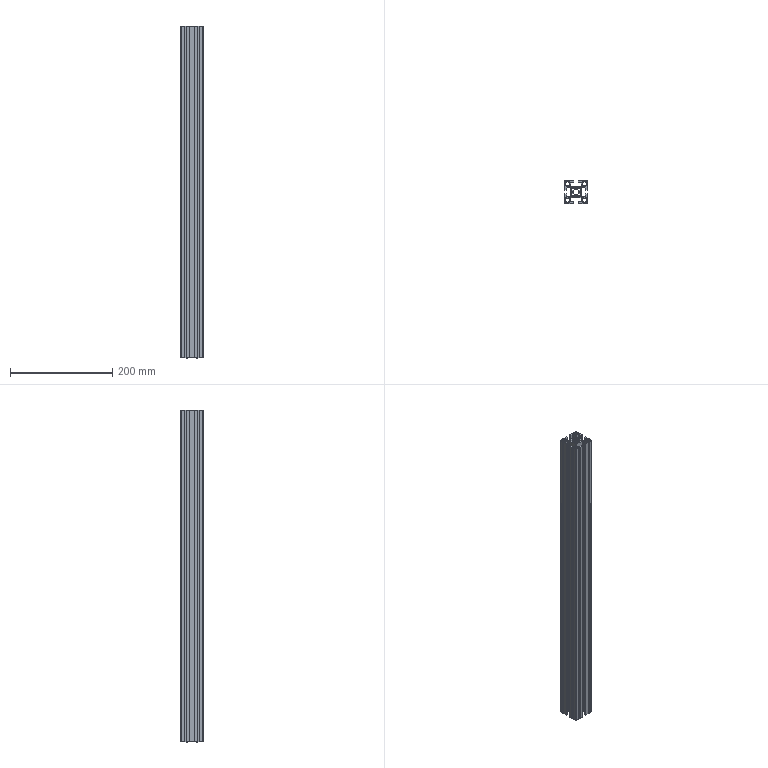Part | STEP file | 4545-650 Al (PC rack 1) | 1 solid | 262 faces | box 45 x 45 x 650 mm | volume 451001 mm3 | plane 186 | cylinder 76 | commonest cylinder face diameters 2 x44 8 x20 12 x8 4 x4